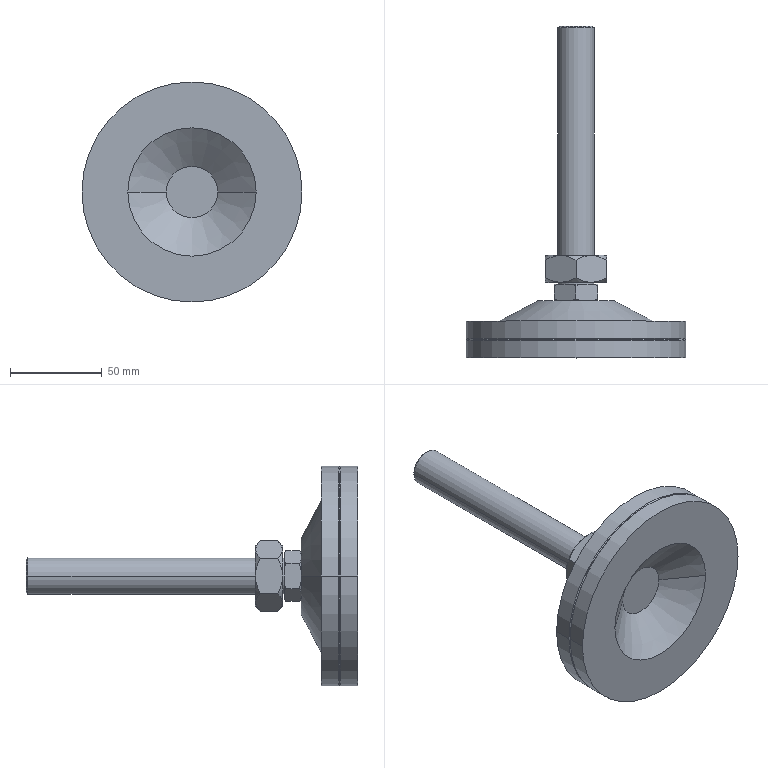Part | SolidWorks | features ICE 2, RevCut 2, Chamfer 1, Revolution 1 | 1 solid | 54 faces | box 120 x 181 x 120 mm | volume 289918 mm3 | cone 26 | plane 20 | cylinder 8 | commonest cylinder face diameters 20 x4 120 x4